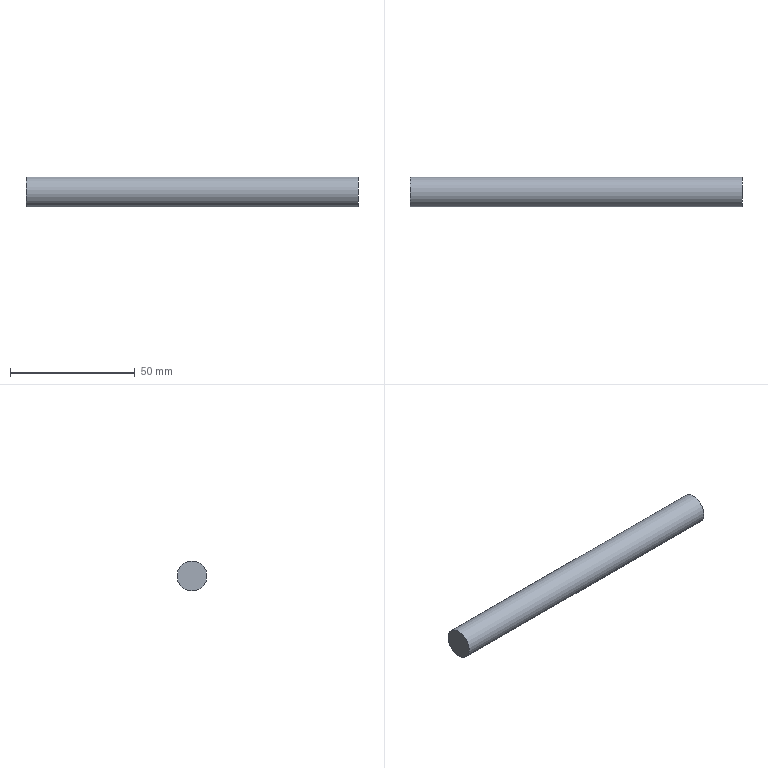Part | STEP file | solid 81 | 1 solid | 3 faces | box 133 x 12 x 12 mm | volume 15042 mm3 | plane 2 | cylinder 1 | commonest cylinder face diameters 12 x1